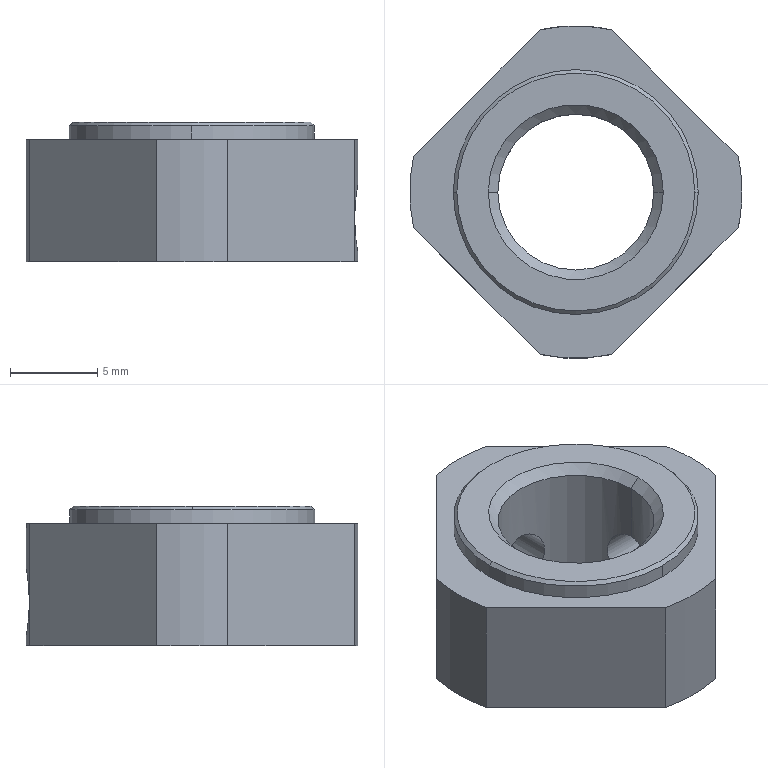Part | SolidWorks | features BaseBody 1 | 1 solid | 30 faces | box 19 x 19 x 8 mm | volume 1253 mm3 | cylinder 13 | cone 10 | plane 7 | commonest cylinder face diameters 19 x5 3.242 x4 8.917 x2 14 x2
STEP:
#1=CARTESIAN_POINT('',(-4.458,0.,0.5415));
#2=VERTEX_POINT('',#1);
#3=CARTESIAN_POINT('',(4.458,0.,0.5415));
#4=VERTEX_POINT('',#3);
#5=CARTESIAN_POINT('',(0.,0.,0.5415));
#6=DIRECTION('',(0.,0.,1.));
#7=DIRECTION('',(1.,0.,0.));
#8=AXIS2_PLACEMENT_3D('',#5,#6,#7);
#9=CIRCLE('',#8,4.458);
#10=EDGE_CURVE('',#2,#4,#9,.T.);
#11=ORIENTED_EDGE('',*,*,#10,.F.);
#12=CARTESIAN_POINT('',(-4.458,0.,7.458));
#13=VERTEX_POINT('',#12);
#14=CARTESIAN_POINT('',(-4.458,0.,0.));
#15=DIRECTION('',(0.,0.,1.));
#16=VECTOR('',#15,1000.);
#17=LINE('',#14,#16);
#18=EDGE_CURVE('',#2,#13,#17,.T.);
#19=ORIENTED_EDGE('',*,*,#18,.T.);
#20=CARTESIAN_POINT('',(4.458,0.,7.458));
#21=VERTEX_POINT('',#20);
#22=CARTESIAN_POINT('',(0.,0.,7.458));
#23=DIRECTION('',(0.,0.,-1.));
#24=DIRECTION('',(1.,0.,0.));
#25=AXIS2_PLACEMENT_3D('',#22,#23,#24);
#26=CIRCLE('',#25,4.458);
#27=EDGE_CURVE('',#21,#13,#26,.T.);
#28=ORIENTED_EDGE('',*,*,#27,.F.);
#29=CARTESIAN_POINT('',(4.459,0.,4.121));
#30=VERTEX_POINT('',#29);
#31=CARTESIAN_POINT('',(4.458,0.,0.));
#32=DIRECTION('',(0.,0.,1.));
#33=VECTOR('',#32,1000.);
#34=LINE('',#31,#33);
#35=EDGE_CURVE('',#30,#21,#34,.T.);
#36=ORIENTED_EDGE('',*,*,#35,.F.);
#37=CARTESIAN_POINT('',(4.459,0.,0.879));
#38=VERTEX_POINT('',#37);
#39=CARTESIAN_POINT('',(4.459,0.,0.879));
#40=CARTESIAN_POINT('',(4.459,-0.1067,0.879));
#41=CARTESIAN_POINT('',(4.455,-0.2126,0.8894));
#42=CARTESIAN_POINT('',(4.44,-0.4226,0.9314));
#43=CARTESIAN_POINT('',(4.429,-0.5256,0.963));
#44=CARTESIAN_POINT('',(4.387,-0.8179,1.085));
#45=CARTESIAN_POINT('',(4.348,-0.9974,1.205));
#46=CARTESIAN_POINT('',(4.289,-1.22,1.427));
#47=CARTESIAN_POINT('',(4.269,-1.288,1.51));
#48=CARTESIAN_POINT('',(4.232,-1.405,1.685));
#49=CARTESIAN_POINT('',(4.215,-1.455,1.778));
#50=CARTESIAN_POINT('',(4.171,-1.578,2.072));
#51=CARTESIAN_POINT('',(4.153,-1.621,2.285));
#52=CARTESIAN_POINT('',(4.153,-1.621,2.608));
#53=CARTESIAN_POINT('',(4.158,-1.61,2.714));
#54=CARTESIAN_POINT('',(4.174,-1.569,2.922));
#55=CARTESIAN_POINT('',(4.185,-1.537,3.026));
#56=CARTESIAN_POINT('',(4.214,-1.455,3.222));
#57=CARTESIAN_POINT('',(4.232,-1.406,3.314));
#58=CARTESIAN_POINT('',(4.269,-1.288,3.489));
#59=CARTESIAN_POINT('',(4.289,-1.221,3.572));
#60=CARTESIAN_POINT('',(4.348,-0.9982,3.794));
#61=CARTESIAN_POINT('',(4.387,-0.819,3.915));
#62=CARTESIAN_POINT('',(4.428,-0.526,4.037));
#63=CARTESIAN_POINT('',(4.44,-0.4226,4.069));
#64=CARTESIAN_POINT('',(4.455,-0.2131,4.11));
#65=CARTESIAN_POINT('',(4.459,-0.1072,4.121));
#66=CARTESIAN_POINT('',(4.459,0.,4.121));
#67=B_SPLINE_CURVE_WITH_KNOTS('',3,(#39,#40,#41,#42,#43,#44,#45,#46,#47,#48,#49,#50,#51,#52,#53,#54,#55,#56,#57,#58,#59,#60,#61,#62,#63,#64,#65,#66),.UNSPECIFIED.,.F.,.F.,(4,2,2,2,2,2,2,2,2,2,2,2,2,4),(0.0001581,0.0004773,0.0007965,0.001435,0.001754,0.002073,0.002712,0.003031,0.00335,0.003669,0.003988,0.004627,0.004946,0.005265),.UNSPECIFIED.);
#68=EDGE_CURVE('',#38,#30,#67,.T.);
#69=ORIENTED_EDGE('',*,*,#68,.F.);
#70=CARTESIAN_POINT('',(4.458,0.,0.));
#71=DIRECTION('',(0.,0.,1.));
#72=VECTOR('',#71,1000.);
#73=LINE('',#70,#72);
#74=EDGE_CURVE('',#4,#38,#73,.T.);
#75=ORIENTED_EDGE('',*,*,#74,.F.);
#76=EDGE_LOOP('',(#11,#19,#28,#36,#69,#75));
#77=FACE_OUTER_BOUND('',#76,.T.);
#78=CARTESIAN_POINT('',(0.,0.,0.));
#79=DIRECTION('',(0.,0.,1.));
#80=DIRECTION('',(1.,0.,0.));
#81=AXIS2_PLACEMENT_3D('',#78,#79,#80);
#82=CYLINDRICAL_SURFACE('',#81,4.458);
#83=ADVANCED_FACE('',(#77),#82,.F.);
#84=ORIENTED_EDGE('',*,*,#68,.T.);
#85=CARTESIAN_POINT('',(9.121,0.,4.121));
#86=VERTEX_POINT('',#85);
#87=CARTESIAN_POINT('',(0.,0.,4.121));
#88=DIRECTION('',(1.,0.,0.));
#89=VECTOR('',#88,1000.);
#90=LINE('',#87,#89);
#91=EDGE_CURVE('',#30,#86,#90,.T.);
#92=ORIENTED_EDGE('',*,*,#91,.T.);
#93=CARTESIAN_POINT('',(9.121,0.,0.879));
#94=VERTEX_POINT('',#93);
#95=CARTESIAN_POINT('',(9.121,0.,2.5));
#96=DIRECTION('',(-1.,0.,0.));
#97=DIRECTION('',(0.,0.,-1.));
#98=AXIS2_PLACEMENT_3D('',#95,#96,#97);
#99=CIRCLE('',#98,1.621);
#100=EDGE_CURVE('',#94,#86,#99,.T.);
#101=ORIENTED_EDGE('',*,*,#100,.F.);
#102=CARTESIAN_POINT('',(0.,0.,0.879));
#103=DIRECTION('',(1.,0.,0.));
#104=VECTOR('',#103,1000.);
#105=LINE('',#102,#104);
#106=EDGE_CURVE('',#38,#94,#105,.T.);
#107=ORIENTED_EDGE('',*,*,#106,.F.);
#108=EDGE_LOOP('',(#84,#92,#101,#107));
#109=FACE_OUTER_BOUND('',#108,.T.);
#110=CARTESIAN_POINT('',(0.,0.,2.5));
#111=DIRECTION('',(1.,0.,0.));
#112=DIRECTION('',(0.,0.,-1.));
#113=AXIS2_PLACEMENT_3D('',#110,#111,#112);
#114=CYLINDRICAL_SURFACE('',#113,1.621);
#115=ADVANCED_FACE('',(#109),#114,.F.);
#116=ORIENTED_EDGE('',*,*,#27,.T.);
#117=CARTESIAN_POINT('',(-5.,0.,8.));
#118=VERTEX_POINT('',#117);
#119=CARTESIAN_POINT('',(-5.,0.,8.));
#120=DIRECTION('',(-0.7071,0.,0.7071));
#121=VECTOR('',#120,1000.);
#122=LINE('',#119,#121);
#123=EDGE_CURVE('',#13,#118,#122,.T.);
#124=ORIENTED_EDGE('',*,*,#123,.T.);
#125=CARTESIAN_POINT('',(5.,0.,8.));
#126=VERTEX_POINT('',#125);
#127=CARTESIAN_POINT('',(0.,0.,8.));
#128=DIRECTION('',(0.,0.,-1.));
#129=DIRECTION('',(1.,0.,0.));
#130=AXIS2_PLACEMENT_3D('',#127,#128,#129);
#131=CIRCLE('',#130,5.);
#132=EDGE_CURVE('',#126,#118,#131,.T.);
#133=ORIENTED_EDGE('',*,*,#132,.F.);
#134=CARTESIAN_POINT('',(5.,0.,8.));
#135=DIRECTION('',(0.7071,0.,0.7071));
#136=VECTOR('',#135,1000.);
#137=LINE('',#134,#136);
#138=EDGE_CURVE('',#21,#126,#137,.T.);
#139=ORIENTED_EDGE('',*,*,#138,.F.);
#140=EDGE_LOOP('',(#116,#124,#133,#139));
#141=FACE_OUTER_BOUND('',#140,.T.);
#142=CARTESIAN_POINT('',(0.,0.,8.));
#143=DIRECTION('',(0.,0.,1.));
#144=DIRECTION('',(1.,0.,0.));
#145=AXIS2_PLACEMENT_3D('',#142,#143,#144);
#146=CONICAL_SURFACE('',#145,5.,0.7854);
#147=ADVANCED_FACE('',(#141),#146,.F.);
#148=CARTESIAN_POINT('',(0.,4.459,4.121));
#149=VERTEX_POINT('',#148);
#150=CARTESIAN_POINT('',(0.,4.459,0.879));
#151=VERTEX_POINT('',#150);
#152=CARTESIAN_POINT('',(0.,4.459,4.121));
#153=CARTESIAN_POINT('',(-0.1067,4.459,4.121));
#154=CARTESIAN_POINT('',(-0.2126,4.455,4.111));
#155=CARTESIAN_POINT('',(-0.4226,4.44,4.069));
#156=CARTESIAN_POINT('',(-0.5256,4.429,4.037));
#157=CARTESIAN_POINT('',(-0.8179,4.387,3.915));
#158=CARTESIAN_POINT('',(-0.9974,4.348,3.795));
#159=CARTESIAN_POINT('',(-1.22,4.289,3.573));
#160=CARTESIAN_POINT('',(-1.288,4.269,3.49));
#161=CARTESIAN_POINT('',(-1.405,4.232,3.315));
#162=CARTESIAN_POINT('',(-1.455,4.215,3.222));
#163=CARTESIAN_POINT('',(-1.578,4.171,2.928));
#164=CARTESIAN_POINT('',(-1.621,4.153,2.715));
#165=CARTESIAN_POINT('',(-1.621,4.153,2.392));
#166=CARTESIAN_POINT('',(-1.61,4.158,2.286));
#167=CARTESIAN_POINT('',(-1.569,4.174,2.078));
#168=CARTESIAN_POINT('',(-1.537,4.185,1.974));
#169=CARTESIAN_POINT('',(-1.455,4.214,1.778));
#170=CARTESIAN_POINT('',(-1.406,4.232,1.686));
#171=CARTESIAN_POINT('',(-1.288,4.269,1.511));
#172=CARTESIAN_POINT('',(-1.221,4.289,1.428));
#173=CARTESIAN_POINT('',(-0.9982,4.348,1.206));
#174=CARTESIAN_POINT('',(-0.819,4.387,1.085));
#175=CARTESIAN_POINT('',(-0.526,4.428,0.9631));
#176=CARTESIAN_POINT('',(-0.4226,4.44,0.9314));
#177=CARTESIAN_POINT('',(-0.2131,4.455,0.8895));
#178=CARTESIAN_POINT('',(-0.1072,4.459,0.879));
#179=CARTESIAN_POINT('',(0.,4.459,0.879));
#180=B_SPLINE_CURVE_WITH_KNOTS('',3,(#152,#153,#154,#155,#156,#157,#158,#159,#160,#161,#162,#163,#164,#165,#166,#167,#168,#169,#170,#171,#172,#173,#174,#175,#176,#177,#178,#179),.UNSPECIFIED.,.F.,.F.,(4,2,2,2,2,2,2,2,2,2,2,2,2,4),(0.0001581,0.0004773,0.0007965,0.001435,0.001754,0.002073,0.002712,0.003031,0.00335,0.003669,0.003988,0.004627,0.004946,0.005265),.UNSPECIFIED.);
#181=EDGE_CURVE('',#149,#151,#180,.T.);
#182=ORIENTED_EDGE('',*,*,#181,.T.);
#183=CARTESIAN_POINT('',(0.,9.121,0.879));
#184=VERTEX_POINT('',#183);
#185=CARTESIAN_POINT('',(0.,0.,0.879));
#186=DIRECTION('',(0.,1.,0.));
#187=VECTOR('',#186,1000.);
#188=LINE('',#185,#187);
#189=EDGE_CURVE('',#151,#184,#188,.T.);
#190=ORIENTED_EDGE('',*,*,#189,.T.);
#191=CARTESIAN_POINT('',(0.,9.121,4.121));
#192=VERTEX_POINT('',#191);
#193=CARTESIAN_POINT('',(0.,9.121,2.5));
#194=DIRECTION('',(0.,-1.,0.));
#195=DIRECTION('',(0.,0.,1.));
#196=AXIS2_PLACEMENT_3D('',#193,#194,#195);
#197=CIRCLE('',#196,1.621);
#198=EDGE_CURVE('',#192,#184,#197,.T.);
#199=ORIENTED_EDGE('',*,*,#198,.F.);
#200=CARTESIAN_POINT('',(0.,0.,4.121));
#201=DIRECTION('',(0.,1.,0.));
#202=VECTOR('',#201,1000.);
#203=LINE('',#200,#202);
#204=EDGE_CURVE('',#149,#192,#203,.T.);
#205=ORIENTED_EDGE('',*,*,#204,.F.);
#206=EDGE_LOOP('',(#182,#190,#199,#205));
#207=FACE_OUTER_BOUND('',#206,.T.);
#208=CARTESIAN_POINT('',(0.,0.,2.5));
#209=DIRECTION('',(0.,1.,0.));
#210=DIRECTION('',(0.,0.,1.));
#211=AXIS2_PLACEMENT_3D('',#208,#209,#210);
#212=CYLINDRICAL_SURFACE('',#211,1.621);
#213=ADVANCED_FACE('',(#207),#212,.F.);
#214=ORIENTED_EDGE('',*,*,#10,.T.);
#215=CARTESIAN_POINT('',(5.,0.,0.));
#216=VERTEX_POINT('',#215);
#217=CARTESIAN_POINT('',(5.,0.,0.));
#218=DIRECTION('',(0.7071,0.,-0.7071));
#219=VECTOR('',#218,1000.);
#220=LINE('',#217,#219);
#221=EDGE_CURVE('',#4,#216,#220,.T.);
#222=ORIENTED_EDGE('',*,*,#221,.T.);
#223=CARTESIAN_POINT('',(-5.,0.,0.));
#224=VERTEX_POINT('',#223);
#225=CARTESIAN_POINT('',(0.,0.,0.));
#226=DIRECTION('',(0.,0.,1.));
#227=DIRECTION('',(-1.,0.,0.));
#228=AXIS2_PLACEMENT_3D('',#225,#226,#227);
#229=CIRCLE('',#228,5.);
#230=EDGE_CURVE('',#224,#216,#229,.T.);
#231=ORIENTED_EDGE('',*,*,#230,.F.);
#232=CARTESIAN_POINT('',(-5.,0.,0.));
#233=DIRECTION('',(-0.7071,0.,-0.7071));
#234=VECTOR('',#233,1000.);
#235=LINE('',#232,#234);
#236=EDGE_CURVE('',#2,#224,#235,.T.);
#237=ORIENTED_EDGE('',*,*,#236,.F.);
#238=EDGE_LOOP('',(#214,#222,#231,#237));
#239=FACE_OUTER_BOUND('',#238,.T.);
#240=CARTESIAN_POINT('',(0.,0.,0.));
#241=DIRECTION('',(0.,0.,-1.));
#242=DIRECTION('',(-1.,0.,0.));
#243=AXIS2_PLACEMENT_3D('',#240,#241,#242);
#244=CONICAL_SURFACE('',#243,5.,0.7854);
#245=ADVANCED_FACE('',(#239),#244,.F.);
#246=ORIENTED_EDGE('',*,*,#100,.T.);
#247=CARTESIAN_POINT('',(9.5,0.,4.5));
#248=VERTEX_POINT('',#247);
#249=CARTESIAN_POINT('',(9.504,0.,4.504));
#250=DIRECTION('',(0.7071,0.,0.7071));
#251=VECTOR('',#250,1000.);
#252=LINE('',#249,#251);
#253=EDGE_CURVE('',#86,#248,#252,.T.);
#254=ORIENTED_EDGE('',*,*,#253,.T.);
#255=CARTESIAN_POINT('',(9.5,0.,0.5));
#256=VERTEX_POINT('',#255);
#257=CARTESIAN_POINT('',(9.5,0.,0.5));
#258=CARTESIAN_POINT('',(9.5,-0.1257,0.5));
#259=CARTESIAN_POINT('',(9.497,-0.2523,0.5147));
#260=CARTESIAN_POINT('',(9.488,-0.495,0.5707));
#261=CARTESIAN_POINT('',(9.481,-0.6136,0.6124));
#262=CARTESIAN_POINT('',(9.463,-0.841,0.7214));
#263=CARTESIAN_POINT('',(9.453,-0.9466,0.787));
#264=CARTESIAN_POINT('',(9.431,-1.143,0.9383));
#265=CARTESIAN_POINT('',(9.42,-1.235,1.025));
#266=CARTESIAN_POINT('',(9.397,-1.4,1.214));
#267=CARTESIAN_POINT('',(9.386,-1.472,1.315));
#268=CARTESIAN_POINT('',(9.365,-1.597,1.529));
#269=CARTESIAN_POINT('',(9.356,-1.651,1.644));
#270=CARTESIAN_POINT('',(9.34,-1.737,1.879));
#271=CARTESIAN_POINT('',(9.334,-1.769,2.));
#272=CARTESIAN_POINT('',(9.326,-1.812,2.246));
#273=CARTESIAN_POINT('',(9.323,-1.823,2.373));
#274=CARTESIAN_POINT('',(9.323,-1.823,2.623));
#275=CARTESIAN_POINT('',(9.325,-1.813,2.747));
#276=CARTESIAN_POINT('',(9.334,-1.77,2.994));
#277=CARTESIAN_POINT('',(9.34,-1.738,3.117));
#278=CARTESIAN_POINT('',(9.363,-1.61,3.469));
#279=CARTESIAN_POINT('',(9.385,-1.482,3.69));
#280=CARTESIAN_POINT('',(9.431,-1.156,4.067));
#281=CARTESIAN_POINT('',(9.455,-0.9544,4.224));
#282=CARTESIAN_POINT('',(9.489,-0.5022,4.441));
#283=CARTESIAN_POINT('',(9.5,-0.2512,4.5));
#284=CARTESIAN_POINT('',(9.5,0.,4.5));
#285=B_SPLINE_CURVE_WITH_KNOTS('',3,(#257,#258,#259,#260,#261,#262,#263,#264,#265,#266,#267,#268,#269,#270,#271,#272,#273,#274,#275,#276,#277,#278,#279,#280,#281,#282,#283,#284),.UNSPECIFIED.,.F.,.F.,(4,2,2,2,2,2,2,2,2,2,2,2,2,4),(0.004283,0.004658,0.005033,0.005408,0.005783,0.006158,0.006533,0.006908,0.007283,0.007659,0.008034,0.008784,0.009534,0.01028),.UNSPECIFIED.);
#286=EDGE_CURVE('',#256,#248,#285,.T.);
#287=ORIENTED_EDGE('',*,*,#286,.F.);
#288=CARTESIAN_POINT('',(9.504,0.,0.496));
#289=DIRECTION('',(0.7071,0.,-0.7071));
#290=VECTOR('',#289,1000.);
#291=LINE('',#288,#290);
#292=EDGE_CURVE('',#94,#256,#291,.T.);
#293=ORIENTED_EDGE('',*,*,#292,.F.);
#294=EDGE_LOOP('',(#246,#254,#287,#293));
#295=FACE_OUTER_BOUND('',#294,.T.);
#296=CARTESIAN_POINT('',(9.504,0.,2.5));
#297=DIRECTION('',(1.,0.,0.));
#298=DIRECTION('',(0.,0.,-1.));
#299=AXIS2_PLACEMENT_3D('',#296,#297,#298);
#300=CONICAL_SURFACE('',#299,2.004,0.7854);
#301=ADVANCED_FACE('',(#295),#300,.F.);
#302=ORIENTED_EDGE('',*,*,#198,.T.);
#303=CARTESIAN_POINT('',(0.,9.5,0.5));
#304=VERTEX_POINT('',#303);
#305=CARTESIAN_POINT('',(0.,9.503,0.4965));
#306=DIRECTION('',(0.,0.7071,-0.7071));
#307=VECTOR('',#306,1000.);
#308=LINE('',#305,#307);
#309=EDGE_CURVE('',#184,#304,#308,.T.);
#310=ORIENTED_EDGE('',*,*,#309,.T.);
#311=CARTESIAN_POINT('',(0.,9.5,4.5));
#312=VERTEX_POINT('',#311);
#313=CARTESIAN_POINT('',(0.,9.5,4.5));
#314=CARTESIAN_POINT('',(-0.2502,9.5,4.5));
#315=CARTESIAN_POINT('',(-0.5019,9.489,4.441));
#316=CARTESIAN_POINT('',(-0.8382,9.464,4.28));
#317=CARTESIAN_POINT('',(-0.9459,9.453,4.214));
#318=CARTESIAN_POINT('',(-1.145,9.431,4.061));
#319=CARTESIAN_POINT('',(-1.235,9.42,3.975));
#320=CARTESIAN_POINT('',(-1.398,9.397,3.788));
#321=CARTESIAN_POINT('',(-1.472,9.386,3.685));
#322=CARTESIAN_POINT('',(-1.598,9.365,3.469));
#323=CARTESIAN_POINT('',(-1.651,9.356,3.357));
#324=CARTESIAN_POINT('',(-1.736,9.34,3.122));
#325=CARTESIAN_POINT('',(-1.769,9.334,2.999));
#326=CARTESIAN_POINT('',(-1.812,9.326,2.753));
#327=CARTESIAN_POINT('',(-1.823,9.323,2.628));
#328=CARTESIAN_POINT('',(-1.824,9.323,2.378));
#329=CARTESIAN_POINT('',(-1.813,9.325,2.251));
#330=CARTESIAN_POINT('',(-1.77,9.334,2.005));
#331=CARTESIAN_POINT('',(-1.738,9.34,1.884));
#332=CARTESIAN_POINT('',(-1.653,9.355,1.648));
#333=CARTESIAN_POINT('',(-1.599,9.365,1.533));
#334=CARTESIAN_POINT('',(-1.474,9.385,1.318));
#335=CARTESIAN_POINT('',(-1.401,9.396,1.216));
#336=CARTESIAN_POINT('',(-1.236,9.42,1.026));
#337=CARTESIAN_POINT('',(-1.145,9.431,0.9402));
#338=CARTESIAN_POINT('',(-0.9478,9.453,0.7877));
#339=CARTESIAN_POINT('',(-0.8396,9.464,0.7207));
#340=CARTESIAN_POINT('',(-0.5014,9.489,0.5587));
#341=CARTESIAN_POINT('',(-0.2502,9.5,0.5));
#342=CARTESIAN_POINT('',(0.,9.5,0.5));
#343=B_SPLINE_CURVE_WITH_KNOTS('',3,(#313,#314,#315,#316,#317,#318,#319,#320,#321,#322,#323,#324,#325,#326,#327,#328,#329,#330,#331,#332,#333,#334,#335,#336,#337,#338,#339,#340,#341,#342),.UNSPECIFIED.,.F.,.F.,(4,2,2,2,2,2,2,2,2,2,2,2,2,2,4),(0.00115,0.001906,0.002284,0.002662,0.00304,0.003418,0.003796,0.004174,0.004552,0.00493,0.005308,0.005686,0.006064,0.006442,0.007198),.UNSPECIFIED.);
#344=EDGE_CURVE('',#312,#304,#343,.T.);
#345=ORIENTED_EDGE('',*,*,#344,.F.);
#346=CARTESIAN_POINT('',(0.,9.503,4.503));
#347=DIRECTION('',(0.,0.7071,0.7071));
#348=VECTOR('',#347,1000.);
#349=LINE('',#346,#348);
#350=EDGE_CURVE('',#192,#312,#349,.T.);
#351=ORIENTED_EDGE('',*,*,#350,.F.);
#352=EDGE_LOOP('',(#302,#310,#345,#351));
#353=FACE_OUTER_BOUND('',#352,.T.);
#354=CARTESIAN_POINT('',(0.,9.503,2.5));
#355=DIRECTION('',(0.,1.,0.));
#356=DIRECTION('',(0.,0.,1.));
#357=AXIS2_PLACEMENT_3D('',#354,#355,#356);
#358=CONICAL_SURFACE('',#357,2.003,0.7854);
#359=ADVANCED_FACE('',(#353),#358,.F.);
#360=CARTESIAN_POINT('',(9.28,-2.034,0.));
#361=VERTEX_POINT('',#360);
#362=CARTESIAN_POINT('',(9.5,0.,0.));
#363=VERTEX_POINT('',#362);
#364=CARTESIAN_POINT('',(0.,0.,0.));
#365=DIRECTION('',(0.,0.,1.));
#366=DIRECTION('',(1.,0.,0.));
#367=AXIS2_PLACEMENT_3D('',#364,#365,#366);
#368=CIRCLE('',#367,9.5);
#369=EDGE_CURVE('',#361,#363,#368,.T.);
#370=ORIENTED_EDGE('',*,*,#369,.T.);
#371=CARTESIAN_POINT('',(9.5,0.,7.));
#372=DIRECTION('',(0.,0.,1.));
#373=VECTOR('',#372,1000.);
#374=LINE('',#371,#373);
#375=EDGE_CURVE('',#363,#256,#374,.T.);
#376=ORIENTED_EDGE('',*,*,#375,.T.);
#377=ORIENTED_EDGE('',*,*,#286,.T.);
#378=CARTESIAN_POINT('',(9.5,0.,7.));
#379=VERTEX_POINT('',#378);
#380=CARTESIAN_POINT('',(9.5,0.,7.));
#381=DIRECTION('',(0.,0.,1.));
#382=VECTOR('',#381,1000.);
#383=LINE('',#380,#382);
#384=EDGE_CURVE('',#248,#379,#383,.T.);
#385=ORIENTED_EDGE('',*,*,#384,.T.);
#386=CARTESIAN_POINT('',(9.28,-2.034,7.));
#387=VERTEX_POINT('',#386);
#388=CARTESIAN_POINT('',(0.,0.,7.));
#389=DIRECTION('',(0.,0.,-1.));
#390=DIRECTION('',(1.,0.,0.));
#391=AXIS2_PLACEMENT_3D('',#388,#389,#390);
#392=CIRCLE('',#391,9.5);
#393=EDGE_CURVE('',#379,#387,#392,.T.);
#394=ORIENTED_EDGE('',*,*,#393,.T.);
#395=CARTESIAN_POINT('',(9.28,-2.034,7.));
#396=DIRECTION('',(0.,0.,-1.));
#397=VECTOR('',#396,1000.);
#398=LINE('',#395,#397);
#399=EDGE_CURVE('',#387,#361,#398,.T.);
#400=ORIENTED_EDGE('',*,*,#399,.T.);
#401=EDGE_LOOP('',(#370,#376,#377,#385,#394,#400));
#402=FACE_OUTER_BOUND('',#401,.T.);
#403=CARTESIAN_POINT('',(0.,0.,7.));
#404=DIRECTION('',(0.,0.,1.));
#405=DIRECTION('',(1.,0.,0.));
#406=AXIS2_PLACEMENT_3D('',#403,#404,#405);
#407=CYLINDRICAL_SURFACE('',#406,9.5);
#408=ADVANCED_FACE('',(#402),#407,.T.);
#409=CARTESIAN_POINT('',(-6.8,0.,8.));
#410=VERTEX_POINT('',#409);
#411=CARTESIAN_POINT('',(6.8,0.,8.));
#412=VERTEX_POINT('',#411);
#413=CARTESIAN_POINT('',(0.,0.,8.));
#414=DIRECTION('',(0.,0.,-1.));
#415=DIRECTION('',(-1.,0.,0.));
#416=AXIS2_PLACEMENT_3D('',#413,#414,#415);
#417=CIRCLE('',#416,6.8);
#418=EDGE_CURVE('',#410,#412,#417,.T.);
#419=ORIENTED_EDGE('',*,*,#418,.T.);
#420=CARTESIAN_POINT('',(7.,0.,7.8));
#421=VERTEX_POINT('',#420);
#422=CARTESIAN_POINT('',(7.,0.,7.8));
#423=DIRECTION('',(0.7071,0.,-0.7071));
#424=VECTOR('',#423,1000.);
#425=LINE('',#422,#424);
#426=EDGE_CURVE('',#412,#421,#425,.T.);
#427=ORIENTED_EDGE('',*,*,#426,.T.);
#428=CARTESIAN_POINT('',(0.,7.,7.8));
#429=VERTEX_POINT('',#428);
#430=CARTESIAN_POINT('',(0.,0.,7.8));
#431=DIRECTION('',(0.,0.,1.));
#432=DIRECTION('',(0.,1.,0.));
#433=AXIS2_PLACEMENT_3D('',#430,#431,#432);
#434=CIRCLE('',#433,7.);
#435=EDGE_CURVE('',#421,#429,#434,.T.);
#436=ORIENTED_EDGE('',*,*,#435,.T.);
#437=CARTESIAN_POINT('',(-7.,0.,7.8));
#438=VERTEX_POINT('',#437);
#439=CARTESIAN_POINT('',(0.,0.,7.8));
#440=DIRECTION('',(0.,0.,1.));
#441=DIRECTION('',(0.,1.,0.));
#442=AXIS2_PLACEMENT_3D('',#439,#440,#441);
#443=CIRCLE('',#442,7.);
#444=EDGE_CURVE('',#429,#438,#443,.T.);
#445=ORIENTED_EDGE('',*,*,#444,.T.);
#446=CARTESIAN_POINT('',(-7.,0.,7.8));
#447=DIRECTION('',(-0.7071,0.,-0.7071));
#448=VECTOR('',#447,1000.);
#449=LINE('',#446,#448);
#450=EDGE_CURVE('',#410,#438,#449,.T.);
#451=ORIENTED_EDGE('',*,*,#450,.F.);
#452=EDGE_LOOP('',(#419,#427,#436,#445,#451));
#453=FACE_OUTER_BOUND('',#452,.T.);
#454=CARTESIAN_POINT('',(0.,0.,7.8));
#455=DIRECTION('',(0.,0.,-1.));
#456=DIRECTION('',(-1.,0.,0.));
#457=AXIS2_PLACEMENT_3D('',#454,#455,#456);
#458=CONICAL_SURFACE('',#457,7.,0.7854);
#459=ADVANCED_FACE('',(#453),#458,.T.);
#460=CARTESIAN_POINT('',(0.,7.,7.));
#461=VERTEX_POINT('',#460);
#462=CARTESIAN_POINT('',(0.,-7.,7.));
#463=VERTEX_POINT('',#462);
#464=CARTESIAN_POINT('',(0.,0.,7.));
#465=DIRECTION('',(0.,0.,-1.));
#466=DIRECTION('',(0.,-1.,0.));
#467=AXIS2_PLACEMENT_3D('',#464,#465,#466);
#468=CIRCLE('',#467,7.);
#469=EDGE_CURVE('',#461,#463,#468,.T.);
#470=ORIENTED_EDGE('',*,*,#469,.F.);
#471=CARTESIAN_POINT('',(0.,7.,0.));
#472=DIRECTION('',(0.,0.,1.));
#473=VECTOR('',#472,1000.);
#474=LINE('',#471,#473);
#475=EDGE_CURVE('',#461,#429,#474,.T.);
#476=ORIENTED_EDGE('',*,*,#475,.T.);
#477=ORIENTED_EDGE('',*,*,#435,.F.);
#478=CARTESIAN_POINT('',(0.,-7.,7.8));
#479=VERTEX_POINT('',#478);
#480=CARTESIAN_POINT('',(0.,0.,7.8));
#481=DIRECTION('',(0.,0.,1.));
#482=DIRECTION('',(0.,1.,0.));
#483=AXIS2_PLACEMENT_3D('',#480,#481,#482);
#484=CIRCLE('',#483,7.);
#485=EDGE_CURVE('',#479,#421,#484,.T.);
#486=ORIENTED_EDGE('',*,*,#485,.F.);
#487=CARTESIAN_POINT('',(0.,-7.,0.));
#488=DIRECTION('',(0.,0.,1.));
#489=VECTOR('',#488,1000.);
#490=LINE('',#487,#489);
#491=EDGE_CURVE('',#463,#479,#490,.T.);
#492=ORIENTED_EDGE('',*,*,#491,.F.);
#493=EDGE_LOOP('',(#470,#476,#477,#486,#492));
#494=FACE_OUTER_BOUND('',#493,.T.);
#495=CARTESIAN_POINT('',(0.,0.,0.));
#496=DIRECTION('',(0.,0.,1.));
#497=DIRECTION('',(0.,-1.,0.));
#498=AXIS2_PLACEMENT_3D('',#495,#496,#497);
#499=CYLINDRICAL_SURFACE('',#498,7.);
#500=ADVANCED_FACE('',(#494),#499,.T.);
#501=ORIENTED_EDGE('',*,*,#18,.F.);
#502=CARTESIAN_POINT('',(0.,0.,0.5415));
#503=DIRECTION('',(0.,0.,1.));
#504=DIRECTION('',(1.,0.,0.));
#505=AXIS2_PLACEMENT_3D('',#502,#503,#504);
#506=CIRCLE('',#505,4.458);
#507=EDGE_CURVE('',#4,#2,#506,.T.);
#508=ORIENTED_EDGE('',*,*,#507,.F.);
#509=ORIENTED_EDGE('',*,*,#74,.T.);
#510=CARTESIAN_POINT('',(4.459,0.,4.121));
#511=CARTESIAN_POINT('',(4.459,0.1071,4.121));
#512=CARTESIAN_POINT('',(4.455,0.2152,4.11));
#513=CARTESIAN_POINT('',(4.44,0.4234,4.068));
#514=CARTESIAN_POINT('',(4.429,0.5248,4.037));
#515=CARTESIAN_POINT('',(4.387,0.8212,3.914));
#516=CARTESIAN_POINT('',(4.348,0.9974,3.795));
#517=CARTESIAN_POINT('',(4.289,1.221,3.571));
#518=CARTESIAN_POINT('',(4.269,1.288,3.49));
#519=CARTESIAN_POINT('',(4.232,1.405,3.315));
#520=CARTESIAN_POINT('',(4.214,1.456,3.221));
#521=CARTESIAN_POINT('',(4.171,1.578,2.928));
#522=CARTESIAN_POINT('',(4.153,1.621,2.713));
#523=CARTESIAN_POINT('',(4.153,1.621,2.393));
#524=CARTESIAN_POINT('',(4.158,1.61,2.285));
#525=CARTESIAN_POINT('',(4.174,1.568,2.076));
#526=CARTESIAN_POINT('',(4.185,1.537,1.975));
#527=CARTESIAN_POINT('',(4.214,1.456,1.78));
#528=CARTESIAN_POINT('',(4.232,1.405,1.685));
#529=CARTESIAN_POINT('',(4.269,1.288,1.51));
#530=CARTESIAN_POINT('',(4.289,1.222,1.429));
#531=CARTESIAN_POINT('',(4.348,0.9978,1.205));
#532=CARTESIAN_POINT('',(4.387,0.8204,1.086));
#533=CARTESIAN_POINT('',(4.429,0.5253,0.9628));
#534=CARTESIAN_POINT('',(4.44,0.4239,0.9318));
#535=CARTESIAN_POINT('',(4.455,0.2152,0.8898));
#536=CARTESIAN_POINT('',(4.458,0.1067,0.879));
#537=CARTESIAN_POINT('',(4.459,0.,0.879));
#538=B_SPLINE_CURVE_WITH_KNOTS('',3,(#510,#511,#512,#513,#514,#515,#516,#517,#518,#519,#520,#521,#522,#523,#524,#525,#526,#527,#528,#529,#530,#531,#532,#533,#534,#535,#536,#537),.UNSPECIFIED.,.F.,.F.,(4,2,2,2,2,2,2,2,2,2,2,2,2,4),(0.005265,0.005584,0.005903,0.006542,0.006861,0.00718,0.007818,0.008138,0.008457,0.008776,0.009095,0.009733,0.01005,0.01037),.UNSPECIFIED.);
#539=EDGE_CURVE('',#30,#38,#538,.T.);
#540=ORIENTED_EDGE('',*,*,#539,.F.);
#541=ORIENTED_EDGE('',*,*,#35,.T.);
#542=CARTESIAN_POINT('',(0.,0.,7.458));
#543=DIRECTION('',(0.,0.,-1.));
#544=DIRECTION('',(1.,0.,0.));
#545=AXIS2_PLACEMENT_3D('',#542,#543,#544);
#546=CIRCLE('',#545,4.458);
#547=EDGE_CURVE('',#13,#21,#546,.T.);
#548=ORIENTED_EDGE('',*,*,#547,.F.);
#549=EDGE_LOOP('',(#501,#508,#509,#540,#541,#548));
#550=FACE_OUTER_BOUND('',#549,.T.);
#551=ORIENTED_EDGE('',*,*,#181,.F.);
#552=CARTESIAN_POINT('',(0.,4.459,0.879));
#553=CARTESIAN_POINT('',(0.1071,4.459,0.879));
#554=CARTESIAN_POINT('',(0.2152,4.455,0.8898));
#555=CARTESIAN_POINT('',(0.4234,4.44,0.9317));
#556=CARTESIAN_POINT('',(0.5248,4.429,0.9626));
#557=CARTESIAN_POINT('',(0.8212,4.387,1.086));
#558=CARTESIAN_POINT('',(0.9974,4.348,1.205));
#559=CARTESIAN_POINT('',(1.221,4.289,1.429));
#560=CARTESIAN_POINT('',(1.288,4.269,1.51));
#561=CARTESIAN_POINT('',(1.405,4.232,1.685));
#562=CARTESIAN_POINT('',(1.456,4.214,1.779));
#563=CARTESIAN_POINT('',(1.578,4.171,2.072));
#564=CARTESIAN_POINT('',(1.621,4.153,2.287));
#565=CARTESIAN_POINT('',(1.621,4.153,2.607));
#566=CARTESIAN_POINT('',(1.61,4.158,2.715));
#567=CARTESIAN_POINT('',(1.568,4.174,2.924));
#568=CARTESIAN_POINT('',(1.537,4.185,3.025));
#569=CARTESIAN_POINT('',(1.456,4.214,3.22));
#570=CARTESIAN_POINT('',(1.405,4.232,3.315));
#571=CARTESIAN_POINT('',(1.288,4.269,3.49));
#572=CARTESIAN_POINT('',(1.222,4.289,3.571));
#573=CARTESIAN_POINT('',(0.9978,4.348,3.795));
#574=CARTESIAN_POINT('',(0.8204,4.387,3.914));
#575=CARTESIAN_POINT('',(0.5253,4.429,4.037));
#576=CARTESIAN_POINT('',(0.4239,4.44,4.068));
#577=CARTESIAN_POINT('',(0.2152,4.455,4.11));
#578=CARTESIAN_POINT('',(0.1067,4.458,4.121));
#579=CARTESIAN_POINT('',(0.,4.459,4.121));
#580=B_SPLINE_CURVE_WITH_KNOTS('',3,(#552,#553,#554,#555,#556,#557,#558,#559,#560,#561,#562,#563,#564,#565,#566,#567,#568,#569,#570,#571,#572,#573,#574,#575,#576,#577,#578,#579),.UNSPECIFIED.,.F.,.F.,(4,2,2,2,2,2,2,2,2,2,2,2,2,4),(0.005265,0.005584,0.005903,0.006542,0.006861,0.00718,0.007818,0.008138,0.008457,0.008776,0.009095,0.009733,0.01005,0.01037),.UNSPECIFIED.);
#581=EDGE_CURVE('',#151,#149,#580,.T.);
#582=ORIENTED_EDGE('',*,*,#581,.F.);
#583=EDGE_LOOP('',(#551,#582));
#584=FACE_BOUND('',#583,.T.);
#585=CARTESIAN_POINT('',(0.,0.,0.));
#586=DIRECTION('',(0.,0.,1.));
#587=DIRECTION('',(1.,0.,0.));
#588=AXIS2_PLACEMENT_3D('',#585,#586,#587);
#589=CYLINDRICAL_SURFACE('',#588,4.458);
#590=ADVANCED_FACE('',(#550,#584),#589,.F.);
#591=ORIENTED_EDGE('',*,*,#91,.F.);
#592=ORIENTED_EDGE('',*,*,#539,.T.);
#593=ORIENTED_EDGE('',*,*,#106,.T.);
#594=CARTESIAN_POINT('',(9.121,0.,2.5));
#595=DIRECTION('',(-1.,0.,0.));
#596=DIRECTION('',(0.,0.,-1.));
#597=AXIS2_PLACEMENT_3D('',#594,#595,#596);
#598=CIRCLE('',#597,1.621);
#599=EDGE_CURVE('',#86,#94,#598,.T.);
#600=ORIENTED_EDGE('',*,*,#599,.F.);
#601=EDGE_LOOP('',(#591,#592,#593,#600));
#602=FACE_OUTER_BOUND('',#601,.T.);
#603=CARTESIAN_POINT('',(0.,0.,2.5));
#604=DIRECTION('',(1.,0.,0.));
#605=DIRECTION('',(0.,0.,-1.));
#606=AXIS2_PLACEMENT_3D('',#603,#604,#605);
#607=CYLINDRICAL_SURFACE('',#606,1.621);
#608=ADVANCED_FACE('',(#602),#607,.F.);
#609=ORIENTED_EDGE('',*,*,#123,.F.);
#610=ORIENTED_EDGE('',*,*,#547,.T.);
#611=ORIENTED_EDGE('',*,*,#138,.T.);
#612=CARTESIAN_POINT('',(0.,0.,8.));
#613=DIRECTION('',(0.,0.,-1.));
#614=DIRECTION('',(1.,0.,0.));
#615=AXIS2_PLACEMENT_3D('',#612,#613,#614);
#616=CIRCLE('',#615,5.);
#617=EDGE_CURVE('',#118,#126,#616,.T.);
#618=ORIENTED_EDGE('',*,*,#617,.F.);
#619=EDGE_LOOP('',(#609,#610,#611,#618));
#620=FACE_OUTER_BOUND('',#619,.T.);
#621=CARTESIAN_POINT('',(0.,0.,8.));
#622=DIRECTION('',(0.,0.,1.));
#623=DIRECTION('',(1.,0.,0.));
#624=AXIS2_PLACEMENT_3D('',#621,#622,#623);
#625=CONICAL_SURFACE('',#624,5.,0.7854);
#626=ADVANCED_FACE('',(#620),#625,.F.);
#627=ORIENTED_EDGE('',*,*,#189,.F.);
#628=ORIENTED_EDGE('',*,*,#581,.T.);
#629=ORIENTED_EDGE('',*,*,#204,.T.);
#630=CARTESIAN_POINT('',(0.,9.121,2.5));
#631=DIRECTION('',(0.,-1.,0.));
#632=DIRECTION('',(0.,0.,1.));
#633=AXIS2_PLACEMENT_3D('',#630,#631,#632);
#634=CIRCLE('',#633,1.621);
#635=EDGE_CURVE('',#184,#192,#634,.T.);
#636=ORIENTED_EDGE('',*,*,#635,.F.);
#637=EDGE_LOOP('',(#627,#628,#629,#636));
#638=FACE_OUTER_BOUND('',#637,.T.);
#639=CARTESIAN_POINT('',(0.,0.,2.5));
#640=DIRECTION('',(0.,1.,0.));
#641=DIRECTION('',(0.,0.,1.));
#642=AXIS2_PLACEMENT_3D('',#639,#640,#641);
#643=CYLINDRICAL_SURFACE('',#642,1.621);
#644=ADVANCED_FACE('',(#638),#643,.F.);
#645=ORIENTED_EDGE('',*,*,#221,.F.);
#646=ORIENTED_EDGE('',*,*,#507,.T.);
#647=ORIENTED_EDGE('',*,*,#236,.T.);
#648=CARTESIAN_POINT('',(0.,0.,0.));
#649=DIRECTION('',(0.,0.,1.));
#650=DIRECTION('',(-1.,0.,0.));
#651=AXIS2_PLACEMENT_3D('',#648,#649,#650);
#652=CIRCLE('',#651,5.);
#653=EDGE_CURVE('',#216,#224,#652,.T.);
#654=ORIENTED_EDGE('',*,*,#653,.F.);
#655=EDGE_LOOP('',(#645,#646,#647,#654));
#656=FACE_OUTER_BOUND('',#655,.T.);
#657=CARTESIAN_POINT('',(0.,0.,0.));
#658=DIRECTION('',(0.,0.,-1.));
#659=DIRECTION('',(-1.,0.,0.));
#660=AXIS2_PLACEMENT_3D('',#657,#658,#659);
#661=CONICAL_SURFACE('',#660,5.,0.7854);
#662=ADVANCED_FACE('',(#656),#661,.F.);
#663=ORIENTED_EDGE('',*,*,#253,.F.);
#664=ORIENTED_EDGE('',*,*,#599,.T.);
#665=ORIENTED_EDGE('',*,*,#292,.T.);
#666=CARTESIAN_POINT('',(9.5,0.,4.5));
#667=CARTESIAN_POINT('',(9.5,0.1255,4.5));
#668=CARTESIAN_POINT('',(9.498,0.2493,4.486));
#669=CARTESIAN_POINT('',(9.488,0.4933,4.43));
#670=CARTESIAN_POINT('',(9.481,0.6134,4.388));
#671=CARTESIAN_POINT('',(9.455,0.9496,4.227));
#672=CARTESIAN_POINT('',(9.431,1.152,4.07));
#673=CARTESIAN_POINT('',(9.397,1.398,3.788));
#674=CARTESIAN_POINT('',(9.386,1.472,3.685));
#675=CARTESIAN_POINT('',(9.365,1.598,3.47));
#676=CARTESIAN_POINT('',(9.356,1.651,3.357));
#677=CARTESIAN_POINT('',(9.34,1.736,3.121));
#678=CARTESIAN_POINT('',(9.334,1.769,2.999));
#679=CARTESIAN_POINT('',(9.326,1.812,2.753));
#680=CARTESIAN_POINT('',(9.323,1.823,2.629));
#681=CARTESIAN_POINT('',(9.323,1.824,2.377));
#682=CARTESIAN_POINT('',(9.325,1.813,2.251));
#683=CARTESIAN_POINT('',(9.334,1.77,2.005));
#684=CARTESIAN_POINT('',(9.34,1.738,1.884));
#685=CARTESIAN_POINT('',(9.363,1.609,1.528));
#686=CARTESIAN_POINT('',(9.385,1.483,1.31));
#687=CARTESIAN_POINT('',(9.42,1.236,1.026));
#688=CARTESIAN_POINT('',(9.431,1.146,0.9404));
#689=CARTESIAN_POINT('',(9.453,0.9474,0.7875));
#690=CARTESIAN_POINT('',(9.464,0.8395,0.7207));
#691=CARTESIAN_POINT('',(9.481,0.6144,0.6128));
#692=CARTESIAN_POINT('',(9.488,0.4947,0.5706));
#693=CARTESIAN_POINT('',(9.498,0.2497,0.5142));
#694=CARTESIAN_POINT('',(9.5,0.1256,0.5));
#695=CARTESIAN_POINT('',(9.5,0.,0.5));
#696=B_SPLINE_CURVE_WITH_KNOTS('',3,(#666,#667,#668,#669,#670,#671,#672,#673,#674,#675,#676,#677,#678,#679,#680,#681,#682,#683,#684,#685,#686,#687,#688,#689,#690,#691,#692,#693,#694,#695),.UNSPECIFIED.,.F.,.F.,(4,2,2,2,2,2,2,2,2,2,2,2,2,2,4),(0.01028,0.01066,0.01103,0.01178,0.01216,0.01253,0.01291,0.01328,0.01366,0.01403,0.01478,0.01516,0.01553,0.01591,0.01628),.UNSPECIFIED.);
#697=EDGE_CURVE('',#248,#256,#696,.T.);
#698=ORIENTED_EDGE('',*,*,#697,.F.);
#699=EDGE_LOOP('',(#663,#664,#665,#698));
#700=FACE_OUTER_BOUND('',#699,.T.);
#701=CARTESIAN_POINT('',(9.504,0.,2.5));
#702=DIRECTION('',(1.,0.,0.));
#703=DIRECTION('',(0.,0.,-1.));
#704=AXIS2_PLACEMENT_3D('',#701,#702,#703);
#705=CONICAL_SURFACE('',#704,2.004,0.7854);
#706=ADVANCED_FACE('',(#700),#705,.F.);
#707=ORIENTED_EDGE('',*,*,#132,.T.);
#708=ORIENTED_EDGE('',*,*,#617,.T.);
#709=EDGE_LOOP('',(#707,#708));
#710=FACE_BOUND('',#709,.T.);
#711=ORIENTED_EDGE('',*,*,#418,.F.);
#712=CARTESIAN_POINT('',(0.,0.,8.));
#713=DIRECTION('',(0.,0.,-1.));
#714=DIRECTION('',(-1.,0.,0.));
#715=AXIS2_PLACEMENT_3D('',#712,#713,#714);
#716=CIRCLE('',#715,6.8);
#717=EDGE_CURVE('',#412,#410,#716,.T.);
#718=ORIENTED_EDGE('',*,*,#717,.F.);
#719=EDGE_LOOP('',(#711,#718));
#720=FACE_OUTER_BOUND('',#719,.T.);
#721=CARTESIAN_POINT('',(0.,0.,8.));
#722=DIRECTION('',(0.,0.,-1.));
#723=DIRECTION('',(0.,1.,0.));
#724=AXIS2_PLACEMENT_3D('',#721,#722,#723);
#725=PLANE('',#724);
#726=ADVANCED_FACE('',(#710,#720),#725,.F.);
#727=ORIENTED_EDGE('',*,*,#309,.F.);
#728=ORIENTED_EDGE('',*,*,#635,.T.);
#729=ORIENTED_EDGE('',*,*,#350,.T.);
#730=CARTESIAN_POINT('',(0.,9.5,0.5));
#731=CARTESIAN_POINT('',(0.1251,9.5,0.5));
#732=CARTESIAN_POINT('',(0.2523,9.497,0.5147));
#733=CARTESIAN_POINT('',(0.4954,9.488,0.5708));
#734=CARTESIAN_POINT('',(0.6128,9.481,0.6121));
#735=CARTESIAN_POINT('',(0.8394,9.464,0.7205));
#736=CARTESIAN_POINT('',(0.9465,9.453,0.787));
#737=CARTESIAN_POINT('',(1.143,9.432,0.9381));
#738=CARTESIAN_POINT('',(1.233,9.42,1.023));
#739=CARTESIAN_POINT('',(1.482,9.385,1.308));
#740=CARTESIAN_POINT('',(1.607,9.363,1.524));
#741=CARTESIAN_POINT('',(1.78,9.332,1.997));
#742=CARTESIAN_POINT('',(1.823,9.323,2.244));
#743=CARTESIAN_POINT('',(1.824,9.323,2.622));
#744=CARTESIAN_POINT('',(1.813,9.325,2.746));
#745=CARTESIAN_POINT('',(1.771,9.334,2.992));
#746=CARTESIAN_POINT('',(1.738,9.34,3.115));
#747=CARTESIAN_POINT('',(1.653,9.355,3.35));
#748=CARTESIAN_POINT('',(1.601,9.364,3.463));
#749=CARTESIAN_POINT('',(1.476,9.385,3.679));
#750=CARTESIAN_POINT('',(1.402,9.396,3.783));
#751=CARTESIAN_POINT('',(1.157,9.431,4.065));
#752=CARTESIAN_POINT('',(0.9564,9.454,4.223));
#753=CARTESIAN_POINT('',(0.6145,9.481,4.387));
#754=CARTESIAN_POINT('',(0.4963,9.488,4.429));
#755=CARTESIAN_POINT('',(0.2523,9.497,4.485));
#756=CARTESIAN_POINT('',(0.1251,9.5,4.5));
#757=CARTESIAN_POINT('',(0.,9.5,4.5));
#758=B_SPLINE_CURVE_WITH_KNOTS('',3,(#730,#731,#732,#733,#734,#735,#736,#737,#738,#739,#740,#741,#742,#743,#744,#745,#746,#747,#748,#749,#750,#751,#752,#753,#754,#755,#756,#757),.UNSPECIFIED.,.F.,.F.,(4,2,2,2,2,2,2,2,2,2,2,2,2,4),(0.007198,0.007576,0.007954,0.008332,0.00871,0.009466,0.01022,0.0106,0.01098,0.01136,0.01173,0.01249,0.01287,0.01325),.UNSPECIFIED.);
#759=EDGE_CURVE('',#304,#312,#758,.T.);
#760=ORIENTED_EDGE('',*,*,#759,.F.);
#761=EDGE_LOOP('',(#727,#728,#729,#760));
#762=FACE_OUTER_BOUND('',#761,.T.);
#763=CARTESIAN_POINT('',(0.,9.503,2.5));
#764=DIRECTION('',(0.,1.,0.));
#765=DIRECTION('',(0.,0.,1.));
#766=AXIS2_PLACEMENT_3D('',#763,#764,#765);
#767=CONICAL_SURFACE('',#766,2.003,0.7854);
#768=ADVANCED_FACE('',(#762),#767,.F.);
#769=CARTESIAN_POINT('',(2.034,9.28,0.));
#770=VERTEX_POINT('',#769);
#771=CARTESIAN_POINT('',(-2.034,9.28,0.));
#772=VERTEX_POINT('',#771);
#773=CARTESIAN_POINT('',(0.,0.,0.));
#774=DIRECTION('',(0.,0.,1.));
#775=DIRECTION('',(1.,0.,0.));
#776=AXIS2_PLACEMENT_3D('',#773,#774,#775);
#777=CIRCLE('',#776,9.5);
#778=EDGE_CURVE('',#770,#772,#777,.T.);
#779=ORIENTED_EDGE('',*,*,#778,.F.);
#780=CARTESIAN_POINT('',(9.28,2.034,0.));
#781=VERTEX_POINT('',#780);
#782=CARTESIAN_POINT('',(9.28,2.034,0.));
#783=DIRECTION('',(-0.7071,0.7071,0.));
#784=VECTOR('',#783,1000.);
#785=LINE('',#782,#784);
#786=EDGE_CURVE('',#781,#770,#785,.T.);
#787=ORIENTED_EDGE('',*,*,#786,.F.);
#788=CARTESIAN_POINT('',(0.,0.,0.));
#789=DIRECTION('',(0.,0.,1.));
#790=DIRECTION('',(1.,0.,0.));
#791=AXIS2_PLACEMENT_3D('',#788,#789,#790);
#792=CIRCLE('',#791,9.5);
#793=EDGE_CURVE('',#363,#781,#792,.T.);
#794=ORIENTED_EDGE('',*,*,#793,.F.);
#795=ORIENTED_EDGE('',*,*,#369,.F.);
#796=CARTESIAN_POINT('',(2.034,-9.28,0.));
#797=VERTEX_POINT('',#796);
#798=CARTESIAN_POINT('',(2.034,-9.28,0.));
#799=DIRECTION('',(0.7071,0.7071,0.));
#800=VECTOR('',#799,1000.);
#801=LINE('',#798,#800);
#802=EDGE_CURVE('',#797,#361,#801,.T.);
#803=ORIENTED_EDGE('',*,*,#802,.F.);
#804=CARTESIAN_POINT('',(-2.034,-9.28,0.));
#805=VERTEX_POINT('',#804);
#806=CARTESIAN_POINT('',(0.,0.,0.));
#807=DIRECTION('',(0.,0.,1.));
#808=DIRECTION('',(1.,0.,0.));
#809=AXIS2_PLACEMENT_3D('',#806,#807,#808);
#810=CIRCLE('',#809,9.5);
#811=EDGE_CURVE('',#805,#797,#810,.T.);
#812=ORIENTED_EDGE('',*,*,#811,.F.);
#813=CARTESIAN_POINT('',(-9.28,-2.034,0.));
#814=VERTEX_POINT('',#813);
#815=CARTESIAN_POINT('',(-9.28,-2.034,0.));
#816=DIRECTION('',(0.7071,-0.7071,0.));
#817=VECTOR('',#816,1000.);
#818=LINE('',#815,#817);
#819=EDGE_CURVE('',#814,#805,#818,.T.);
#820=ORIENTED_EDGE('',*,*,#819,.F.);
#821=CARTESIAN_POINT('',(-9.28,2.034,0.));
#822=VERTEX_POINT('',#821);
#823=CARTESIAN_POINT('',(0.,0.,0.));
#824=DIRECTION('',(0.,0.,1.));
#825=DIRECTION('',(1.,0.,0.));
#826=AXIS2_PLACEMENT_3D('',#823,#824,#825);
#827=CIRCLE('',#826,9.5);
#828=EDGE_CURVE('',#822,#814,#827,.T.);
#829=ORIENTED_EDGE('',*,*,#828,.F.);
#830=CARTESIAN_POINT('',(-2.034,9.28,0.));
#831=DIRECTION('',(-0.7071,-0.7071,0.));
#832=VECTOR('',#831,1000.);
#833=LINE('',#830,#832);
#834=EDGE_CURVE('',#772,#822,#833,.T.);
#835=ORIENTED_EDGE('',*,*,#834,.F.);
#836=EDGE_LOOP('',(#779,#787,#794,#795,#803,#812,#820,#829,#835));
#837=FACE_OUTER_BOUND('',#836,.T.);
#838=ORIENTED_EDGE('',*,*,#230,.T.);
#839=ORIENTED_EDGE('',*,*,#653,.T.);
#840=EDGE_LOOP('',(#838,#839));
#841=FACE_BOUND('',#840,.T.);
#842=CARTESIAN_POINT('',(0.,0.,0.));
#843=DIRECTION('',(0.,0.,1.));
#844=DIRECTION('',(1.,0.,0.));
#845=AXIS2_PLACEMENT_3D('',#842,#843,#844);
#846=PLANE('',#845);
#847=ADVANCED_FACE('',(#837,#841),#846,.F.);
#848=ORIENTED_EDGE('',*,*,#375,.F.);
#849=ORIENTED_EDGE('',*,*,#793,.T.);
#850=CARTESIAN_POINT('',(9.28,2.034,7.));
#851=VERTEX_POINT('',#850);
#852=CARTESIAN_POINT('',(9.28,2.034,7.));
#853=DIRECTION('',(0.,0.,1.));
#854=VECTOR('',#853,1000.);
#855=LINE('',#852,#854);
#856=EDGE_CURVE('',#781,#851,#855,.T.);
#857=ORIENTED_EDGE('',*,*,#856,.T.);
#858=CARTESIAN_POINT('',(0.,0.,7.));
#859=DIRECTION('',(0.,0.,-1.));
#860=DIRECTION('',(1.,0.,0.));
#861=AXIS2_PLACEMENT_3D('',#858,#859,#860);
#862=CIRCLE('',#861,9.5);
#863=EDGE_CURVE('',#851,#379,#862,.T.);
#864=ORIENTED_EDGE('',*,*,#863,.T.);
#865=ORIENTED_EDGE('',*,*,#384,.F.);
#866=ORIENTED_EDGE('',*,*,#697,.T.);
#867=EDGE_LOOP('',(#848,#849,#857,#864,#865,#866));
#868=FACE_OUTER_BOUND('',#867,.T.);
#869=CARTESIAN_POINT('',(0.,0.,7.));
#870=DIRECTION('',(0.,0.,1.));
#871=DIRECTION('',(1.,0.,0.));
#872=AXIS2_PLACEMENT_3D('',#869,#870,#871);
#873=CYLINDRICAL_SURFACE('',#872,9.5);
#874=ADVANCED_FACE('',(#868),#873,.T.);
#875=ORIENTED_EDGE('',*,*,#426,.F.);
#876=ORIENTED_EDGE('',*,*,#717,.T.);
#877=ORIENTED_EDGE('',*,*,#450,.T.);
#878=CARTESIAN_POINT('',(0.,0.,7.8));
#879=DIRECTION('',(0.,0.,1.));
#880=DIRECTION('',(0.,1.,0.));
#881=AXIS2_PLACEMENT_3D('',#878,#879,#880);
#882=CIRCLE('',#881,7.);
#883=EDGE_CURVE('',#438,#479,#882,.T.);
#884=ORIENTED_EDGE('',*,*,#883,.T.);
#885=ORIENTED_EDGE('',*,*,#485,.T.);
#886=EDGE_LOOP('',(#875,#876,#877,#884,#885));
#887=FACE_OUTER_BOUND('',#886,.T.);
#888=CARTESIAN_POINT('',(0.,0.,7.8));
#889=DIRECTION('',(0.,0.,-1.));
#890=DIRECTION('',(-1.,0.,0.));
#891=AXIS2_PLACEMENT_3D('',#888,#889,#890);
#892=CONICAL_SURFACE('',#891,7.,0.7854);
#893=ADVANCED_FACE('',(#887),#892,.T.);
#894=ORIENTED_EDGE('',*,*,#344,.T.);
#895=ORIENTED_EDGE('',*,*,#759,.T.);
#896=EDGE_LOOP('',(#894,#895));
#897=FACE_BOUND('',#896,.T.);
#898=CARTESIAN_POINT('',(-2.034,9.28,7.));
#899=VERTEX_POINT('',#898);
#900=CARTESIAN_POINT('',(2.034,9.28,7.));
#901=VERTEX_POINT('',#900);
#902=CARTESIAN_POINT('',(0.,0.,7.));
#903=DIRECTION('',(0.,0.,-1.));
#904=DIRECTION('',(1.,0.,0.));
#905=AXIS2_PLACEMENT_3D('',#902,#903,#904);
#906=CIRCLE('',#905,9.5);
#907=EDGE_CURVE('',#899,#901,#906,.T.);
#908=ORIENTED_EDGE('',*,*,#907,.T.);
#909=CARTESIAN_POINT('',(2.034,9.28,7.));
#910=DIRECTION('',(0.,0.,-1.));
#911=VECTOR('',#910,1000.);
#912=LINE('',#909,#911);
#913=EDGE_CURVE('',#901,#770,#912,.T.);
#914=ORIENTED_EDGE('',*,*,#913,.T.);
#915=ORIENTED_EDGE('',*,*,#778,.T.);
#916=CARTESIAN_POINT('',(-2.034,9.28,7.));
#917=DIRECTION('',(0.,0.,1.));
#918=VECTOR('',#917,1000.);
#919=LINE('',#916,#918);
#920=EDGE_CURVE('',#772,#899,#919,.T.);
#921=ORIENTED_EDGE('',*,*,#920,.T.);
#922=EDGE_LOOP('',(#908,#914,#915,#921));
#923=FACE_OUTER_BOUND('',#922,.T.);
#924=CARTESIAN_POINT('',(0.,0.,7.));
#925=DIRECTION('',(0.,0.,1.));
#926=DIRECTION('',(1.,0.,0.));
#927=AXIS2_PLACEMENT_3D('',#924,#925,#926);
#928=CYLINDRICAL_SURFACE('',#927,9.5);
#929=ADVANCED_FACE('',(#897,#923),#928,.T.);
#930=CARTESIAN_POINT('',(-9.28,2.034,7.));
#931=VERTEX_POINT('',#930);
#932=CARTESIAN_POINT('',(-9.28,2.034,7.));
#933=DIRECTION('',(0.,0.,-1.));
#934=VECTOR('',#933,1000.);
#935=LINE('',#932,#934);
#936=EDGE_CURVE('',#931,#822,#935,.T.);
#937=ORIENTED_EDGE('',*,*,#936,.F.);
#938=CARTESIAN_POINT('',(-2.034,9.28,7.));
#939=DIRECTION('',(-0.7071,-0.7071,0.));
#940=VECTOR('',#939,1000.);
#941=LINE('',#938,#940);
#942=EDGE_CURVE('',#899,#931,#941,.T.);
#943=ORIENTED_EDGE('',*,*,#942,.F.);
#944=ORIENTED_EDGE('',*,*,#920,.F.);
#945=ORIENTED_EDGE('',*,*,#834,.T.);
#946=EDGE_LOOP('',(#937,#943,#944,#945));
#947=FACE_OUTER_BOUND('',#946,.T.);
#948=CARTESIAN_POINT('',(-2.034,9.28,7.));
#949=DIRECTION('',(0.7071,-0.7071,0.));
#950=DIRECTION('',(0.7071,0.7071,0.));
#951=AXIS2_PLACEMENT_3D('',#948,#949,#950);
#952=PLANE('',#951);
#953=ADVANCED_FACE('',(#947),#952,.F.);
#954=ORIENTED_EDGE('',*,*,#913,.F.);
#955=CARTESIAN_POINT('',(9.28,2.034,7.));
#956=DIRECTION('',(-0.7071,0.7071,0.));
#957=VECTOR('',#956,1000.);
#958=LINE('',#955,#957);
#959=EDGE_CURVE('',#851,#901,#958,.T.);
#960=ORIENTED_EDGE('',*,*,#959,.F.);
#961=ORIENTED_EDGE('',*,*,#856,.F.);
#962=ORIENTED_EDGE('',*,*,#786,.T.);
#963=EDGE_LOOP('',(#954,#960,#961,#962));
#964=FACE_OUTER_BOUND('',#963,.T.);
#965=CARTESIAN_POINT('',(9.28,2.034,7.));
#966=DIRECTION('',(-0.7071,-0.7071,0.));
#967=DIRECTION('',(0.7071,-0.7071,0.));
#968=AXIS2_PLACEMENT_3D('',#965,#966,#967);
#969=PLANE('',#968);
#970=ADVANCED_FACE('',(#964),#969,.F.);
#971=ORIENTED_EDGE('',*,*,#399,.F.);
#972=CARTESIAN_POINT('',(2.034,-9.28,7.));
#973=VERTEX_POINT('',#972);
#974=CARTESIAN_POINT('',(2.034,-9.28,7.));
#975=DIRECTION('',(0.7071,0.7071,0.));
#976=VECTOR('',#975,1000.);
#977=LINE('',#974,#976);
#978=EDGE_CURVE('',#973,#387,#977,.T.);
#979=ORIENTED_EDGE('',*,*,#978,.F.);
#980=CARTESIAN_POINT('',(2.034,-9.28,7.));
#981=DIRECTION('',(0.,0.,1.));
#982=VECTOR('',#981,1000.);
#983=LINE('',#980,#982);
#984=EDGE_CURVE('',#797,#973,#983,.T.);
#985=ORIENTED_EDGE('',*,*,#984,.F.);
#986=ORIENTED_EDGE('',*,*,#802,.T.);
#987=EDGE_LOOP('',(#971,#979,#985,#986));
#988=FACE_OUTER_BOUND('',#987,.T.);
#989=CARTESIAN_POINT('',(2.034,-9.28,7.));
#990=DIRECTION('',(-0.7071,0.7071,0.));
#991=DIRECTION('',(-0.7071,-0.7071,0.));
#992=AXIS2_PLACEMENT_3D('',#989,#990,#991);
#993=PLANE('',#992);
#994=ADVANCED_FACE('',(#988),#993,.F.);
#995=CARTESIAN_POINT('',(-2.034,-9.28,7.));
#996=VERTEX_POINT('',#995);
#997=CARTESIAN_POINT('',(0.,0.,7.));
#998=DIRECTION('',(0.,0.,-1.));
#999=DIRECTION('',(1.,0.,0.));
#1000=AXIS2_PLACEMENT_3D('',#997,#998,#999);
#1001=CIRCLE('',#1000,9.5);
#1002=EDGE_CURVE('',#973,#996,#1001,.T.);
#1003=ORIENTED_EDGE('',*,*,#1002,.T.);
#1004=CARTESIAN_POINT('',(-2.034,-9.28,7.));
#1005=DIRECTION('',(0.,0.,-1.));
#1006=VECTOR('',#1005,1000.);
#1007=LINE('',#1004,#1006);
#1008=EDGE_CURVE('',#996,#805,#1007,.T.);
#1009=ORIENTED_EDGE('',*,*,#1008,.T.);
#1010=ORIENTED_EDGE('',*,*,#811,.T.);
#1011=ORIENTED_EDGE('',*,*,#984,.T.);
#1012=EDGE_LOOP('',(#1003,#1009,#1010,#1011));
#1013=FACE_OUTER_BOUND('',#1012,.T.);
#1014=CARTESIAN_POINT('',(0.,0.,7.));
#1015=DIRECTION('',(0.,0.,1.));
#1016=DIRECTION('',(1.,0.,0.));
#1017=AXIS2_PLACEMENT_3D('',#1014,#1015,#1016);
#1018=CYLINDRICAL_SURFACE('',#1017,9.5);
#1019=ADVANCED_FACE('',(#1013),#1018,.T.);
#1020=ORIENTED_EDGE('',*,*,#1008,.F.);
#1021=CARTESIAN_POINT('',(-9.28,-2.034,7.));
#1022=VERTEX_POINT('',#1021);
#1023=CARTESIAN_POINT('',(-9.28,-2.034,7.));
#1024=DIRECTION('',(0.7071,-0.7071,0.));
#1025=VECTOR('',#1024,1000.);
#1026=LINE('',#1023,#1025);
#1027=EDGE_CURVE('',#1022,#996,#1026,.T.);
#1028=ORIENTED_EDGE('',*,*,#1027,.F.);
#1029=CARTESIAN_POINT('',(-9.28,-2.034,7.));
#1030=DIRECTION('',(0.,0.,1.));
#1031=VECTOR('',#1030,1000.);
#1032=LINE('',#1029,#1031);
#1033=EDGE_CURVE('',#814,#1022,#1032,.T.);
#1034=ORIENTED_EDGE('',*,*,#1033,.F.);
#1035=ORIENTED_EDGE('',*,*,#819,.T.);
#1036=EDGE_LOOP('',(#1020,#1028,#1034,#1035));
#1037=FACE_OUTER_BOUND('',#1036,.T.);
#1038=CARTESIAN_POINT('',(-9.28,-2.034,7.));
#1039=DIRECTION('',(0.7071,0.7071,0.));
#1040=DIRECTION('',(-0.7071,0.7071,0.));
#1041=AXIS2_PLACEMENT_3D('',#1038,#1039,#1040);
#1042=PLANE('',#1041);
#1043=ADVANCED_FACE('',(#1037),#1042,.F.);
#1044=CARTESIAN_POINT('',(0.,0.,7.));
#1045=DIRECTION('',(0.,0.,-1.));
#1046=DIRECTION('',(1.,0.,0.));
#1047=AXIS2_PLACEMENT_3D('',#1044,#1045,#1046);
#1048=CIRCLE('',#1047,9.5);
#1049=EDGE_CURVE('',#1022,#931,#1048,.T.);
#1050=ORIENTED_EDGE('',*,*,#1049,.T.);
#1051=ORIENTED_EDGE('',*,*,#936,.T.);
#1052=ORIENTED_EDGE('',*,*,#828,.T.);
#1053=ORIENTED_EDGE('',*,*,#1033,.T.);
#1054=EDGE_LOOP('',(#1050,#1051,#1052,#1053));
#1055=FACE_OUTER_BOUND('',#1054,.T.);
#1056=CARTESIAN_POINT('',(0.,0.,7.));
#1057=DIRECTION('',(0.,0.,1.));
#1058=DIRECTION('',(1.,0.,0.));
#1059=AXIS2_PLACEMENT_3D('',#1056,#1057,#1058);
#1060=CYLINDRICAL_SURFACE('',#1059,9.5);
#1061=ADVANCED_FACE('',(#1055),#1060,.T.);
#1062=ORIENTED_EDGE('',*,*,#959,.T.);
#1063=ORIENTED_EDGE('',*,*,#907,.F.);
#1064=ORIENTED_EDGE('',*,*,#942,.T.);
#1065=ORIENTED_EDGE('',*,*,#1049,.F.);
#1066=ORIENTED_EDGE('',*,*,#1027,.T.);
#1067=ORIENTED_EDGE('',*,*,#1002,.F.);
#1068=ORIENTED_EDGE('',*,*,#978,.T.);
#1069=ORIENTED_EDGE('',*,*,#393,.F.);
#1070=ORIENTED_EDGE('',*,*,#863,.F.);
#1071=EDGE_LOOP('',(#1062,#1063,#1064,#1065,#1066,#1067,#1068,#1069,#1070));
#1072=FACE_OUTER_BOUND('',#1071,.T.);
#1073=CARTESIAN_POINT('',(0.,0.,7.));
#1074=DIRECTION('',(0.,0.,-1.));
#1075=DIRECTION('',(0.,-1.,0.));
#1076=AXIS2_PLACEMENT_3D('',#1073,#1074,#1075);
#1077=CIRCLE('',#1076,7.);
#1078=EDGE_CURVE('',#463,#461,#1077,.T.);
#1079=ORIENTED_EDGE('',*,*,#1078,.T.);
#1080=ORIENTED_EDGE('',*,*,#469,.T.);
#1081=EDGE_LOOP('',(#1079,#1080));
#1082=FACE_BOUND('',#1081,.T.);
#1083=CARTESIAN_POINT('',(0.,0.,7.));
#1084=DIRECTION('',(0.,0.,1.));
#1085=DIRECTION('',(1.,0.,0.));
#1086=AXIS2_PLACEMENT_3D('',#1083,#1084,#1085);
#1087=PLANE('',#1086);
#1088=ADVANCED_FACE('',(#1072,#1082),#1087,.T.);
#1089=ORIENTED_EDGE('',*,*,#475,.F.);
#1090=ORIENTED_EDGE('',*,*,#1078,.F.);
#1091=ORIENTED_EDGE('',*,*,#491,.T.);
#1092=ORIENTED_EDGE('',*,*,#883,.F.);
#1093=ORIENTED_EDGE('',*,*,#444,.F.);
#1094=EDGE_LOOP('',(#1089,#1090,#1091,#1092,#1093));
#1095=FACE_OUTER_BOUND('',#1094,.T.);
#1096=CARTESIAN_POINT('',(0.,0.,0.));
#1097=DIRECTION('',(0.,0.,1.));
#1098=DIRECTION('',(0.,-1.,0.));
#1099=AXIS2_PLACEMENT_3D('',#1096,#1097,#1098);
#1100=CYLINDRICAL_SURFACE('',#1099,7.);
#1101=ADVANCED_FACE('',(#1095),#1100,.T.);
#1102=CLOSED_SHELL('',(#83,#115,#147,#213,#245,#301,#359,#408,#459,#500,#590,#608,#626,#644,#662,#706,#726,#768,#847,#874,#893,#929,#953,#970,#994,#1019,#1043,#1061,#1088,#1101));
#1103=MANIFOLD_SOLID_BREP('',#1102);
#1104=CARTESIAN_POINT('',(0.,0.,0.));
#1105=DIRECTION('',(0.,0.,1.));
#1106=DIRECTION('',(1.,0.,0.));
#1107=AXIS2_PLACEMENT_3D('',#1104,#1105,#1106);
#1108=(LENGTH_UNIT()NAMED_UNIT(*)SI_UNIT(.MILLI.,.METRE.));
#1109=UNCERTAINTY_MEASURE_WITH_UNIT(LENGTH_MEASURE(0.00001),#1108,'','');
#1110=(NAMED_UNIT(*)PLANE_ANGLE_UNIT()SI_UNIT($,.RADIAN.));
#1111=(NAMED_UNIT(*)SI_UNIT($,.STERADIAN.)SOLID_ANGLE_UNIT());
#1112=(GEOMETRIC_REPRESENTATION_CONTEXT(3)GLOBAL_UNCERTAINTY_ASSIGNED_CONTEXT((#1109))GLOBAL_UNIT_ASSIGNED_CONTEXT((#1108,#1110,#1111))REPRESENTATION_CONTEXT('',''));
#1113=ADVANCED_BREP_SHAPE_REPRESENTATION('',(#1103,#1107),#1112);